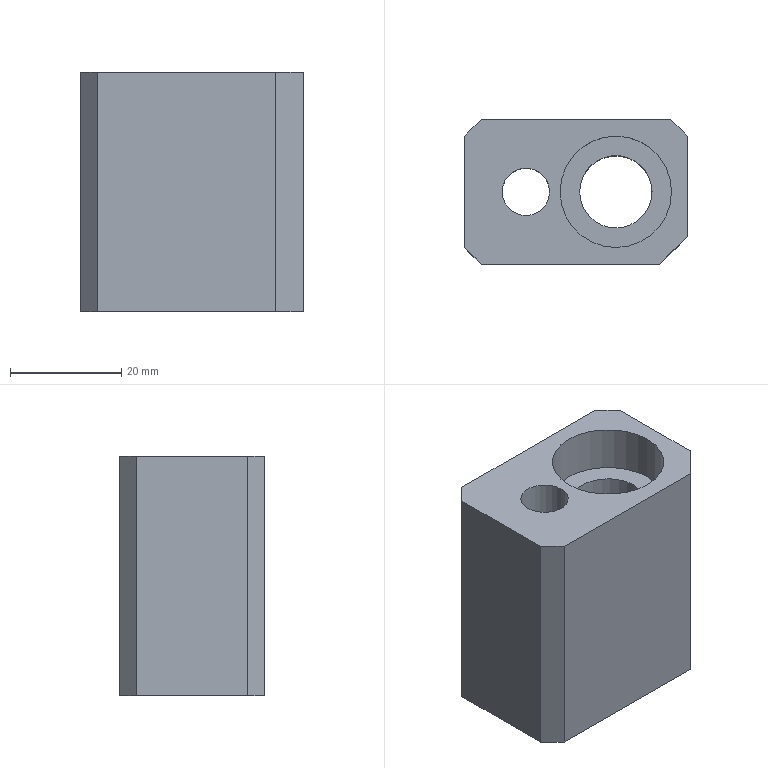Part | NX | features PH-2 2 | 1 solid | 16 faces | box 40 x 26 x 43 mm | volume 32756 mm3 | plane 12 | cylinder 4 | commonest cylinder face diameters 8.5 x1 13.001 x1 14.5 x1 20 x1
STEP:
#1=CARTESIAN_POINT('',(2406.699,-858.122,945.716));
#2=VERTEX_POINT('',#1);
#3=CARTESIAN_POINT('',(2396.699,-858.122,945.716));
#4=DIRECTION('',(0.,0.,-1.));
#5=DIRECTION('',(1.,0.,0.));
#6=AXIS2_PLACEMENT_3D('',#3,#4,#5);
#7=CIRCLE('',#6,10.);
#8=EDGE_CURVE('',#2,#2,#7,.T.);
#9=ORIENTED_EDGE('',*,*,#8,.T.);
#10=EDGE_LOOP('',(#9));
#11=FACE_BOUND('',#10,.T.);
#12=CARTESIAN_POINT('',(2384.799,-858.122,945.716));
#13=VERTEX_POINT('',#12);
#14=CARTESIAN_POINT('',(2380.549,-858.122,945.716));
#15=DIRECTION('',(0.,0.,1.));
#16=DIRECTION('',(1.,0.,0.));
#17=AXIS2_PLACEMENT_3D('',#14,#15,#16);
#18=CIRCLE('',#17,4.25);
#19=EDGE_CURVE('',#13,#13,#18,.T.);
#20=ORIENTED_EDGE('',*,*,#19,.F.);
#21=EDGE_LOOP('',(#20));
#22=FACE_BOUND('',#21,.T.);
#23=CARTESIAN_POINT('',(2404.549,-871.122,945.716));
#24=VERTEX_POINT('',#23);
#25=CARTESIAN_POINT('',(2372.549,-871.122,945.716));
#26=VERTEX_POINT('',#25);
#27=CARTESIAN_POINT('',(2387.049,-871.122,945.716));
#28=DIRECTION('',(-1.,0.,0.));
#29=VECTOR('',#28,1000.);
#30=LINE('',#27,#29);
#31=EDGE_CURVE('',#24,#26,#30,.T.);
#32=ORIENTED_EDGE('',*,*,#31,.F.);
#33=CARTESIAN_POINT('',(2409.549,-866.122,945.716));
#34=VERTEX_POINT('',#33);
#35=CARTESIAN_POINT('',(2402.299,-873.372,945.716));
#36=DIRECTION('',(-0.7071,-0.7071,0.));
#37=VECTOR('',#36,1000.);
#38=LINE('',#35,#37);
#39=EDGE_CURVE('',#24,#34,#38,.F.);
#40=ORIENTED_EDGE('',*,*,#39,.T.);
#41=CARTESIAN_POINT('',(2409.549,-848.122,945.716));
#42=VERTEX_POINT('',#41);
#43=CARTESIAN_POINT('',(2409.549,-858.122,945.716));
#44=DIRECTION('',(0.,-1.,0.));
#45=VECTOR('',#44,1000.);
#46=LINE('',#43,#45);
#47=EDGE_CURVE('',#42,#34,#46,.T.);
#48=ORIENTED_EDGE('',*,*,#47,.F.);
#49=CARTESIAN_POINT('',(2406.549,-845.122,945.716));
#50=VERTEX_POINT('',#49);
#51=CARTESIAN_POINT('',(2403.299,-841.872,945.716));
#52=DIRECTION('',(0.7071,-0.7071,0.));
#53=VECTOR('',#52,1000.);
#54=LINE('',#51,#53);
#55=EDGE_CURVE('',#42,#50,#54,.F.);
#56=ORIENTED_EDGE('',*,*,#55,.T.);
#57=CARTESIAN_POINT('',(2372.549,-845.122,945.716));
#58=VERTEX_POINT('',#57);
#59=CARTESIAN_POINT('',(2387.049,-845.122,945.716));
#60=DIRECTION('',(1.,0.,0.));
#61=VECTOR('',#60,1000.);
#62=LINE('',#59,#61);
#63=EDGE_CURVE('',#58,#50,#62,.T.);
#64=ORIENTED_EDGE('',*,*,#63,.F.);
#65=CARTESIAN_POINT('',(2369.549,-848.122,945.716));
#66=VERTEX_POINT('',#65);
#67=CARTESIAN_POINT('',(2375.799,-841.872,945.716));
#68=DIRECTION('',(0.7071,0.7071,0.));
#69=VECTOR('',#68,1000.);
#70=LINE('',#67,#69);
#71=EDGE_CURVE('',#58,#66,#70,.F.);
#72=ORIENTED_EDGE('',*,*,#71,.T.);
#73=CARTESIAN_POINT('',(2369.549,-868.122,945.716));
#74=VERTEX_POINT('',#73);
#75=CARTESIAN_POINT('',(2369.549,-858.122,945.716));
#76=DIRECTION('',(0.,1.,0.));
#77=VECTOR('',#76,1000.);
#78=LINE('',#75,#77);
#79=EDGE_CURVE('',#74,#66,#78,.T.);
#80=ORIENTED_EDGE('',*,*,#79,.F.);
#81=CARTESIAN_POINT('',(2375.799,-874.372,945.716));
#82=DIRECTION('',(-0.7071,0.7071,0.));
#83=VECTOR('',#82,1000.);
#84=LINE('',#81,#83);
#85=EDGE_CURVE('',#74,#26,#84,.F.);
#86=ORIENTED_EDGE('',*,*,#85,.T.);
#87=EDGE_LOOP('',(#32,#40,#48,#56,#64,#72,#80,#86));
#88=FACE_BOUND('',#87,.T.);
#89=CARTESIAN_POINT('',(2387.049,-858.122,945.716));
#90=DIRECTION('',(0.,0.,1.));
#91=DIRECTION('',(0.,1.,0.));
#92=AXIS2_PLACEMENT_3D('',#89,#90,#91);
#93=PLANE('',#92);
#94=ADVANCED_FACE('',(#11,#22,#88),#93,.T.);
#95=ORIENTED_EDGE('',*,*,#47,.T.);
#96=CARTESIAN_POINT('',(2409.549,-866.122,902.716));
#97=VERTEX_POINT('',#96);
#98=CARTESIAN_POINT('',(2409.549,-866.122,920.716));
#99=DIRECTION('',(0.,0.,-1.));
#100=VECTOR('',#99,1000.);
#101=LINE('',#98,#100);
#102=EDGE_CURVE('',#34,#97,#101,.T.);
#103=ORIENTED_EDGE('',*,*,#102,.T.);
#104=CARTESIAN_POINT('',(2409.549,-848.122,902.716));
#105=VERTEX_POINT('',#104);
#106=CARTESIAN_POINT('',(2409.549,-858.122,902.716));
#107=DIRECTION('',(0.,1.,0.));
#108=VECTOR('',#107,1000.);
#109=LINE('',#106,#108);
#110=EDGE_CURVE('',#97,#105,#109,.T.);
#111=ORIENTED_EDGE('',*,*,#110,.T.);
#112=CARTESIAN_POINT('',(2409.549,-848.122,920.716));
#113=DIRECTION('',(0.,0.,1.));
#114=VECTOR('',#113,1000.);
#115=LINE('',#112,#114);
#116=EDGE_CURVE('',#105,#42,#115,.T.);
#117=ORIENTED_EDGE('',*,*,#116,.T.);
#118=EDGE_LOOP('',(#95,#103,#111,#117));
#119=FACE_BOUND('',#118,.T.);
#120=CARTESIAN_POINT('',(2409.549,-858.122,920.716));
#121=DIRECTION('',(1.,0.,0.));
#122=DIRECTION('',(0.,0.,-1.));
#123=AXIS2_PLACEMENT_3D('',#120,#121,#122);
#124=PLANE('',#123);
#125=ADVANCED_FACE('',(#119),#124,.T.);
#126=CARTESIAN_POINT('',(2372.549,-871.122,902.716));
#127=VERTEX_POINT('',#126);
#128=CARTESIAN_POINT('',(2404.549,-871.122,902.716));
#129=VERTEX_POINT('',#128);
#130=CARTESIAN_POINT('',(2387.049,-871.122,902.716));
#131=DIRECTION('',(1.,0.,0.));
#132=VECTOR('',#131,1000.);
#133=LINE('',#130,#132);
#134=EDGE_CURVE('',#127,#129,#133,.T.);
#135=ORIENTED_EDGE('',*,*,#134,.T.);
#136=CARTESIAN_POINT('',(2404.549,-871.122,920.716));
#137=DIRECTION('',(0.,0.,1.));
#138=VECTOR('',#137,1000.);
#139=LINE('',#136,#138);
#140=EDGE_CURVE('',#129,#24,#139,.T.);
#141=ORIENTED_EDGE('',*,*,#140,.T.);
#142=ORIENTED_EDGE('',*,*,#31,.T.);
#143=CARTESIAN_POINT('',(2372.549,-871.122,920.716));
#144=DIRECTION('',(0.,0.,-1.));
#145=VECTOR('',#144,1000.);
#146=LINE('',#143,#145);
#147=EDGE_CURVE('',#26,#127,#146,.T.);
#148=ORIENTED_EDGE('',*,*,#147,.T.);
#149=EDGE_LOOP('',(#135,#141,#142,#148));
#150=FACE_BOUND('',#149,.T.);
#151=CARTESIAN_POINT('',(2387.049,-871.122,920.716));
#152=DIRECTION('',(0.,-1.,0.));
#153=DIRECTION('',(0.,0.,1.));
#154=AXIS2_PLACEMENT_3D('',#151,#152,#153);
#155=PLANE('',#154);
#156=ADVANCED_FACE('',(#150),#155,.T.);
#157=CARTESIAN_POINT('',(2369.549,-848.122,902.716));
#158=VERTEX_POINT('',#157);
#159=CARTESIAN_POINT('',(2369.549,-868.122,902.716));
#160=VERTEX_POINT('',#159);
#161=CARTESIAN_POINT('',(2369.549,-858.122,902.716));
#162=DIRECTION('',(0.,-1.,0.));
#163=VECTOR('',#162,1000.);
#164=LINE('',#161,#163);
#165=EDGE_CURVE('',#158,#160,#164,.T.);
#166=ORIENTED_EDGE('',*,*,#165,.T.);
#167=CARTESIAN_POINT('',(2369.549,-868.122,920.716));
#168=DIRECTION('',(0.,0.,1.));
#169=VECTOR('',#168,1000.);
#170=LINE('',#167,#169);
#171=EDGE_CURVE('',#160,#74,#170,.T.);
#172=ORIENTED_EDGE('',*,*,#171,.T.);
#173=ORIENTED_EDGE('',*,*,#79,.T.);
#174=CARTESIAN_POINT('',(2369.549,-848.122,920.716));
#175=DIRECTION('',(0.,0.,-1.));
#176=VECTOR('',#175,1000.);
#177=LINE('',#174,#176);
#178=EDGE_CURVE('',#66,#158,#177,.T.);
#179=ORIENTED_EDGE('',*,*,#178,.T.);
#180=EDGE_LOOP('',(#166,#172,#173,#179));
#181=FACE_BOUND('',#180,.T.);
#182=CARTESIAN_POINT('',(2369.549,-858.122,920.716));
#183=DIRECTION('',(-1.,0.,0.));
#184=DIRECTION('',(0.,0.,1.));
#185=AXIS2_PLACEMENT_3D('',#182,#183,#184);
#186=PLANE('',#185);
#187=ADVANCED_FACE('',(#181),#186,.T.);
#188=CARTESIAN_POINT('',(2390.199,-858.122,902.716));
#189=VERTEX_POINT('',#188);
#190=CARTESIAN_POINT('',(2396.699,-858.122,902.716));
#191=DIRECTION('',(0.,0.,-1.));
#192=DIRECTION('',(-1.,0.,0.));
#193=AXIS2_PLACEMENT_3D('',#190,#191,#192);
#194=CIRCLE('',#193,6.5);
#195=EDGE_CURVE('',#189,#189,#194,.T.);
#196=ORIENTED_EDGE('',*,*,#195,.F.);
#197=EDGE_LOOP('',(#196));
#198=FACE_BOUND('',#197,.T.);
#199=CARTESIAN_POINT('',(2373.299,-858.122,902.716));
#200=VERTEX_POINT('',#199);
#201=CARTESIAN_POINT('',(2380.549,-858.122,902.716));
#202=DIRECTION('',(0.,0.,-1.));
#203=DIRECTION('',(-1.,0.,0.));
#204=AXIS2_PLACEMENT_3D('',#201,#202,#203);
#205=CIRCLE('',#204,7.25);
#206=EDGE_CURVE('',#200,#200,#205,.F.);
#207=ORIENTED_EDGE('',*,*,#206,.T.);
#208=EDGE_LOOP('',(#207));
#209=FACE_BOUND('',#208,.T.);
#210=ORIENTED_EDGE('',*,*,#110,.F.);
#211=CARTESIAN_POINT('',(2402.299,-873.372,902.716));
#212=DIRECTION('',(0.7071,0.7071,0.));
#213=VECTOR('',#212,1000.);
#214=LINE('',#211,#213);
#215=EDGE_CURVE('',#97,#129,#214,.F.);
#216=ORIENTED_EDGE('',*,*,#215,.T.);
#217=ORIENTED_EDGE('',*,*,#134,.F.);
#218=CARTESIAN_POINT('',(2373.299,-871.872,902.716));
#219=DIRECTION('',(0.7071,-0.7071,0.));
#220=VECTOR('',#219,1000.);
#221=LINE('',#218,#220);
#222=EDGE_CURVE('',#127,#160,#221,.F.);
#223=ORIENTED_EDGE('',*,*,#222,.T.);
#224=ORIENTED_EDGE('',*,*,#165,.F.);
#225=CARTESIAN_POINT('',(2372.549,-845.122,902.716));
#226=VERTEX_POINT('',#225);
#227=CARTESIAN_POINT('',(2373.299,-844.372,902.716));
#228=DIRECTION('',(-0.7071,-0.7071,0.));
#229=VECTOR('',#228,1000.);
#230=LINE('',#227,#229);
#231=EDGE_CURVE('',#158,#226,#230,.F.);
#232=ORIENTED_EDGE('',*,*,#231,.T.);
#233=CARTESIAN_POINT('',(2406.549,-845.122,902.716));
#234=VERTEX_POINT('',#233);
#235=CARTESIAN_POINT('',(2387.049,-845.122,902.716));
#236=DIRECTION('',(-1.,0.,0.));
#237=VECTOR('',#236,1000.);
#238=LINE('',#235,#237);
#239=EDGE_CURVE('',#234,#226,#238,.T.);
#240=ORIENTED_EDGE('',*,*,#239,.F.);
#241=CARTESIAN_POINT('',(2403.299,-841.872,902.716));
#242=DIRECTION('',(-0.7071,0.7071,0.));
#243=VECTOR('',#242,1000.);
#244=LINE('',#241,#243);
#245=EDGE_CURVE('',#234,#105,#244,.F.);
#246=ORIENTED_EDGE('',*,*,#245,.T.);
#247=EDGE_LOOP('',(#210,#216,#217,#223,#224,#232,#240,#246));
#248=FACE_BOUND('',#247,.T.);
#249=CARTESIAN_POINT('',(2387.049,-858.122,902.716));
#250=DIRECTION('',(0.,0.,-1.));
#251=DIRECTION('',(0.,-1.,0.));
#252=AXIS2_PLACEMENT_3D('',#249,#250,#251);
#253=PLANE('',#252);
#254=ADVANCED_FACE('',(#198,#209,#248),#253,.T.);
#255=ORIENTED_EDGE('',*,*,#239,.T.);
#256=CARTESIAN_POINT('',(2372.549,-845.122,920.716));
#257=DIRECTION('',(0.,0.,1.));
#258=VECTOR('',#257,1000.);
#259=LINE('',#256,#258);
#260=EDGE_CURVE('',#226,#58,#259,.T.);
#261=ORIENTED_EDGE('',*,*,#260,.T.);
#262=ORIENTED_EDGE('',*,*,#63,.T.);
#263=CARTESIAN_POINT('',(2406.549,-845.122,920.716));
#264=DIRECTION('',(0.,0.,-1.));
#265=VECTOR('',#264,1000.);
#266=LINE('',#263,#265);
#267=EDGE_CURVE('',#50,#234,#266,.T.);
#268=ORIENTED_EDGE('',*,*,#267,.T.);
#269=EDGE_LOOP('',(#255,#261,#262,#268));
#270=FACE_BOUND('',#269,.T.);
#271=CARTESIAN_POINT('',(2387.049,-845.122,920.716));
#272=DIRECTION('',(0.,1.,0.));
#273=DIRECTION('',(0.,0.,-1.));
#274=AXIS2_PLACEMENT_3D('',#271,#272,#273);
#275=PLANE('',#274);
#276=ADVANCED_FACE('',(#270),#275,.T.);
#277=ORIENTED_EDGE('',*,*,#231,.F.);
#278=ORIENTED_EDGE('',*,*,#178,.F.);
#279=ORIENTED_EDGE('',*,*,#71,.F.);
#280=ORIENTED_EDGE('',*,*,#260,.F.);
#281=EDGE_LOOP('',(#277,#278,#279,#280));
#282=FACE_BOUND('',#281,.T.);
#283=CARTESIAN_POINT('',(2372.549,-845.122,920.716));
#284=DIRECTION('',(0.7071,-0.7071,0.));
#285=DIRECTION('',(0.7071,0.7071,0.));
#286=AXIS2_PLACEMENT_3D('',#283,#284,#285);
#287=PLANE('',#286);
#288=ADVANCED_FACE('',(#282),#287,.F.);
#289=ORIENTED_EDGE('',*,*,#245,.F.);
#290=ORIENTED_EDGE('',*,*,#267,.F.);
#291=ORIENTED_EDGE('',*,*,#55,.F.);
#292=ORIENTED_EDGE('',*,*,#116,.F.);
#293=EDGE_LOOP('',(#289,#290,#291,#292));
#294=FACE_BOUND('',#293,.T.);
#295=CARTESIAN_POINT('',(2409.549,-848.122,920.716));
#296=DIRECTION('',(-0.7071,-0.7071,0.));
#297=DIRECTION('',(0.7071,-0.7071,0.));
#298=AXIS2_PLACEMENT_3D('',#295,#296,#297);
#299=PLANE('',#298);
#300=ADVANCED_FACE('',(#294),#299,.F.);
#301=ORIENTED_EDGE('',*,*,#222,.F.);
#302=ORIENTED_EDGE('',*,*,#147,.F.);
#303=ORIENTED_EDGE('',*,*,#85,.F.);
#304=ORIENTED_EDGE('',*,*,#171,.F.);
#305=EDGE_LOOP('',(#301,#302,#303,#304));
#306=FACE_BOUND('',#305,.T.);
#307=CARTESIAN_POINT('',(2369.549,-868.122,920.716));
#308=DIRECTION('',(0.7071,0.7071,0.));
#309=DIRECTION('',(-0.7071,0.7071,0.));
#310=AXIS2_PLACEMENT_3D('',#307,#308,#309);
#311=PLANE('',#310);
#312=ADVANCED_FACE('',(#306),#311,.F.);
#313=CARTESIAN_POINT('',(2384.799,-858.122,913.716));
#314=VERTEX_POINT('',#313);
#315=CARTESIAN_POINT('',(2380.549,-858.122,913.716));
#316=DIRECTION('',(0.,0.,1.));
#317=DIRECTION('',(1.,0.,0.));
#318=AXIS2_PLACEMENT_3D('',#315,#316,#317);
#319=CIRCLE('',#318,4.25);
#320=EDGE_CURVE('',#314,#314,#319,.T.);
#321=ORIENTED_EDGE('',*,*,#320,.T.);
#322=EDGE_LOOP('',(#321));
#323=FACE_BOUND('',#322,.T.);
#324=CARTESIAN_POINT('',(2387.799,-858.122,913.716));
#325=VERTEX_POINT('',#324);
#326=CARTESIAN_POINT('',(2380.549,-858.122,913.716));
#327=DIRECTION('',(0.,0.,1.));
#328=DIRECTION('',(1.,0.,0.));
#329=AXIS2_PLACEMENT_3D('',#326,#327,#328);
#330=CIRCLE('',#329,7.25);
#331=EDGE_CURVE('',#325,#325,#330,.T.);
#332=ORIENTED_EDGE('',*,*,#331,.F.);
#333=EDGE_LOOP('',(#332));
#334=FACE_BOUND('',#333,.T.);
#335=CARTESIAN_POINT('',(2380.549,-858.122,913.716));
#336=DIRECTION('',(0.,0.,1.));
#337=DIRECTION('',(1.,0.,0.));
#338=AXIS2_PLACEMENT_3D('',#335,#336,#337);
#339=PLANE('',#338);
#340=ADVANCED_FACE('',(#323,#334),#339,.F.);
#341=ORIENTED_EDGE('',*,*,#206,.F.);
#342=EDGE_LOOP('',(#341));
#343=FACE_BOUND('',#342,.T.);
#344=ORIENTED_EDGE('',*,*,#331,.T.);
#345=EDGE_LOOP('',(#344));
#346=FACE_BOUND('',#345,.T.);
#347=CARTESIAN_POINT('',(2380.549,-858.122,931.716));
#348=DIRECTION('',(0.,0.,-1.));
#349=DIRECTION('',(0.,1.,0.));
#350=AXIS2_PLACEMENT_3D('',#347,#348,#349);
#351=CYLINDRICAL_SURFACE('',#350,7.25);
#352=ADVANCED_FACE('',(#343,#346),#351,.F.);
#353=ORIENTED_EDGE('',*,*,#19,.T.);
#354=EDGE_LOOP('',(#353));
#355=FACE_BOUND('',#354,.T.);
#356=ORIENTED_EDGE('',*,*,#320,.F.);
#357=EDGE_LOOP('',(#356));
#358=FACE_BOUND('',#357,.T.);
#359=CARTESIAN_POINT('',(2380.549,-858.122,946.716));
#360=DIRECTION('',(0.,0.,-1.));
#361=DIRECTION('',(0.,1.,0.));
#362=AXIS2_PLACEMENT_3D('',#359,#360,#361);
#363=CYLINDRICAL_SURFACE('',#362,4.25);
#364=ADVANCED_FACE('',(#355,#358),#363,.F.);
#365=ORIENTED_EDGE('',*,*,#39,.F.);
#366=ORIENTED_EDGE('',*,*,#140,.F.);
#367=ORIENTED_EDGE('',*,*,#215,.F.);
#368=ORIENTED_EDGE('',*,*,#102,.F.);
#369=EDGE_LOOP('',(#365,#366,#367,#368));
#370=FACE_BOUND('',#369,.T.);
#371=CARTESIAN_POINT('',(2409.549,-866.122,920.716));
#372=DIRECTION('',(-0.7071,0.7071,0.));
#373=DIRECTION('',(0.,0.,-1.));
#374=AXIS2_PLACEMENT_3D('',#371,#372,#373);
#375=PLANE('',#374);
#376=ADVANCED_FACE('',(#370),#375,.F.);
#377=ORIENTED_EDGE('',*,*,#195,.T.);
#378=EDGE_LOOP('',(#377));
#379=FACE_BOUND('',#378,.T.);
#380=CARTESIAN_POINT('',(2390.199,-858.122,937.416));
#381=VERTEX_POINT('',#380);
#382=CARTESIAN_POINT('',(2396.699,-858.122,937.416));
#383=DIRECTION('',(0.,0.,-1.));
#384=DIRECTION('',(-1.,0.,0.));
#385=AXIS2_PLACEMENT_3D('',#382,#383,#384);
#386=CIRCLE('',#385,6.5);
#387=EDGE_CURVE('',#381,#381,#386,.F.);
#388=ORIENTED_EDGE('',*,*,#387,.T.);
#389=EDGE_LOOP('',(#388));
#390=FACE_BOUND('',#389,.T.);
#391=CARTESIAN_POINT('',(2396.699,-858.122,945.716));
#392=DIRECTION('',(0.,0.,-1.));
#393=DIRECTION('',(1.,0.,0.));
#394=AXIS2_PLACEMENT_3D('',#391,#392,#393);
#395=CYLINDRICAL_SURFACE('',#394,6.5);
#396=ADVANCED_FACE('',(#379,#390),#395,.F.);
#397=ORIENTED_EDGE('',*,*,#387,.F.);
#398=EDGE_LOOP('',(#397));
#399=FACE_BOUND('',#398,.T.);
#400=CARTESIAN_POINT('',(2406.699,-858.122,937.416));
#401=VERTEX_POINT('',#400);
#402=CARTESIAN_POINT('',(2396.699,-858.122,937.416));
#403=DIRECTION('',(0.,0.,1.));
#404=DIRECTION('',(1.,0.,0.));
#405=AXIS2_PLACEMENT_3D('',#402,#403,#404);
#406=CIRCLE('',#405,10.);
#407=EDGE_CURVE('',#401,#401,#406,.T.);
#408=ORIENTED_EDGE('',*,*,#407,.T.);
#409=EDGE_LOOP('',(#408));
#410=FACE_BOUND('',#409,.T.);
#411=CARTESIAN_POINT('',(2396.699,-858.122,937.416));
#412=DIRECTION('',(0.,0.,-1.));
#413=DIRECTION('',(-1.,0.,0.));
#414=AXIS2_PLACEMENT_3D('',#411,#412,#413);
#415=PLANE('',#414);
#416=ADVANCED_FACE('',(#399,#410),#415,.F.);
#417=ORIENTED_EDGE('',*,*,#407,.F.);
#418=EDGE_LOOP('',(#417));
#419=FACE_BOUND('',#418,.T.);
#420=ORIENTED_EDGE('',*,*,#8,.F.);
#421=EDGE_LOOP('',(#420));
#422=FACE_BOUND('',#421,.T.);
#423=CARTESIAN_POINT('',(2396.699,-858.122,945.716));
#424=DIRECTION('',(0.,0.,-1.));
#425=DIRECTION('',(1.,0.,0.));
#426=AXIS2_PLACEMENT_3D('',#423,#424,#425);
#427=CYLINDRICAL_SURFACE('',#426,10.);
#428=ADVANCED_FACE('',(#419,#422),#427,.F.);
#429=CLOSED_SHELL('',(#94,#125,#156,#187,#254,#276,#288,#300,#312,#340,#352,#364,#376,#396,#416,#428));
#430=MANIFOLD_SOLID_BREP('',#429);
#431=(LENGTH_UNIT()NAMED_UNIT(*)SI_UNIT(.MILLI.,.METRE.));
#432=UNCERTAINTY_MEASURE_WITH_UNIT(LENGTH_MEASURE(0.00001),#431,'','');
#433=(NAMED_UNIT(*)PLANE_ANGLE_UNIT()SI_UNIT($,.RADIAN.));
#434=(NAMED_UNIT(*)SI_UNIT($,.STERADIAN.)SOLID_ANGLE_UNIT());
#435=(GEOMETRIC_REPRESENTATION_CONTEXT(3)GLOBAL_UNCERTAINTY_ASSIGNED_CONTEXT((#432))GLOBAL_UNIT_ASSIGNED_CONTEXT((#431,#433,#434))REPRESENTATION_CONTEXT('',''));
#436=ADVANCED_BREP_SHAPE_REPRESENTATION('',(#430),#435);